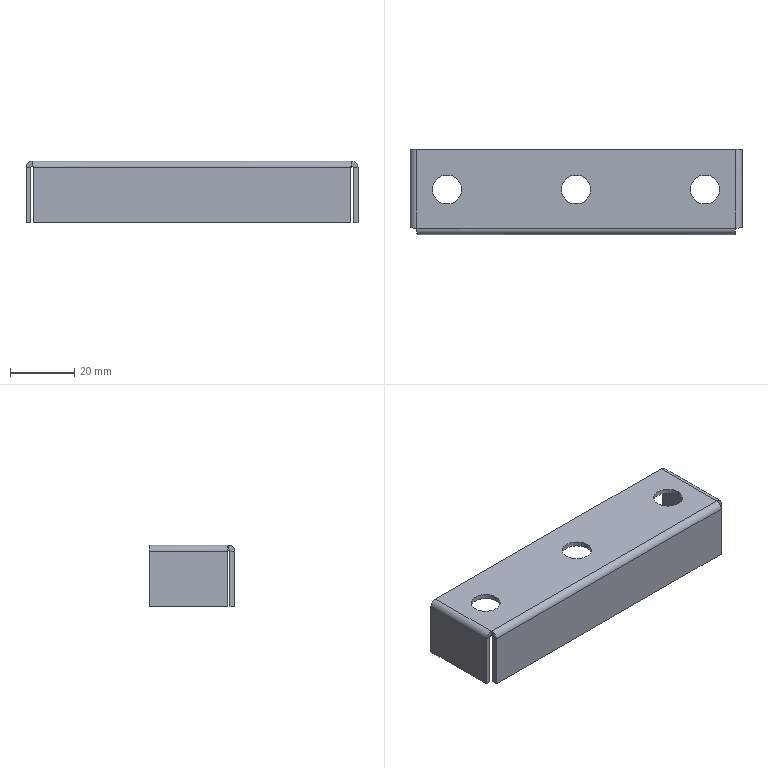Part | SolidWorks | features BaseBody 1 | 1 solid | 36 faces | box 103 x 26.5 x 19.1 mm | volume 7562 mm3 | plane 20 | cylinder 12 | spline 4 | commonest cylinder face diameters 9 x6 1 x3 4 x3
STEP:
#1=CARTESIAN_POINT('',(35.5,0.,-1.5));
#2=VERTEX_POINT('',#1);
#3=CARTESIAN_POINT('',(35.5,0.,0.));
#4=VERTEX_POINT('',#3);
#5=CARTESIAN_POINT('',(35.5,0.,-1.5));
#6=DIRECTION('',(0.,0.,1.));
#7=VECTOR('',#6,1000.);
#8=LINE('',#5,#7);
#9=EDGE_CURVE('',#2,#4,#8,.T.);
#10=ORIENTED_EDGE('',*,*,#9,.F.);
#11=CARTESIAN_POINT('',(44.5,0.,-1.5));
#12=VERTEX_POINT('',#11);
#13=CARTESIAN_POINT('',(40.,0.,-1.5));
#14=DIRECTION('',(0.,0.,1.));
#15=DIRECTION('',(1.,0.,0.));
#16=AXIS2_PLACEMENT_3D('',#13,#14,#15);
#17=CIRCLE('',#16,4.5);
#18=EDGE_CURVE('',#12,#2,#17,.T.);
#19=ORIENTED_EDGE('',*,*,#18,.F.);
#20=CARTESIAN_POINT('',(44.5,0.,0.));
#21=VERTEX_POINT('',#20);
#22=CARTESIAN_POINT('',(44.5,0.,-1.5));
#23=DIRECTION('',(0.,0.,1.));
#24=VECTOR('',#23,1000.);
#25=LINE('',#22,#24);
#26=EDGE_CURVE('',#12,#21,#25,.T.);
#27=ORIENTED_EDGE('',*,*,#26,.T.);
#28=CARTESIAN_POINT('',(40.,0.,0.));
#29=DIRECTION('',(0.,0.,1.));
#30=DIRECTION('',(1.,0.,0.));
#31=AXIS2_PLACEMENT_3D('',#28,#29,#30);
#32=CIRCLE('',#31,4.5);
#33=EDGE_CURVE('',#21,#4,#32,.T.);
#34=ORIENTED_EDGE('',*,*,#33,.T.);
#35=EDGE_LOOP('',(#10,#19,#27,#34));
#36=FACE_OUTER_BOUND('',#35,.T.);
#37=CARTESIAN_POINT('',(40.,0.,-1.5));
#38=DIRECTION('',(0.,0.,1.));
#39=DIRECTION('',(1.,0.,0.));
#40=AXIS2_PLACEMENT_3D('',#37,#38,#39);
#41=CYLINDRICAL_SURFACE('',#40,4.5);
#42=ADVANCED_FACE('',(#36),#41,.F.);
#43=CARTESIAN_POINT('',(-44.5,0.,-1.5));
#44=VERTEX_POINT('',#43);
#45=CARTESIAN_POINT('',(-44.5,0.,0.));
#46=VERTEX_POINT('',#45);
#47=CARTESIAN_POINT('',(-44.5,0.,-1.5));
#48=DIRECTION('',(0.,0.,1.));
#49=VECTOR('',#48,1000.);
#50=LINE('',#47,#49);
#51=EDGE_CURVE('',#44,#46,#50,.T.);
#52=ORIENTED_EDGE('',*,*,#51,.F.);
#53=CARTESIAN_POINT('',(-35.5,0.,-1.5));
#54=VERTEX_POINT('',#53);
#55=CARTESIAN_POINT('',(-40.,0.,-1.5));
#56=DIRECTION('',(0.,0.,1.));
#57=DIRECTION('',(1.,0.,0.));
#58=AXIS2_PLACEMENT_3D('',#55,#56,#57);
#59=CIRCLE('',#58,4.5);
#60=EDGE_CURVE('',#54,#44,#59,.T.);
#61=ORIENTED_EDGE('',*,*,#60,.F.);
#62=CARTESIAN_POINT('',(-35.5,0.,0.));
#63=VERTEX_POINT('',#62);
#64=CARTESIAN_POINT('',(-35.5,0.,-1.5));
#65=DIRECTION('',(0.,0.,1.));
#66=VECTOR('',#65,1000.);
#67=LINE('',#64,#66);
#68=EDGE_CURVE('',#54,#63,#67,.T.);
#69=ORIENTED_EDGE('',*,*,#68,.T.);
#70=CARTESIAN_POINT('',(-40.,0.,0.));
#71=DIRECTION('',(0.,0.,1.));
#72=DIRECTION('',(1.,0.,0.));
#73=AXIS2_PLACEMENT_3D('',#70,#71,#72);
#74=CIRCLE('',#73,4.5);
#75=EDGE_CURVE('',#63,#46,#74,.T.);
#76=ORIENTED_EDGE('',*,*,#75,.T.);
#77=EDGE_LOOP('',(#52,#61,#69,#76));
#78=FACE_OUTER_BOUND('',#77,.T.);
#79=CARTESIAN_POINT('',(-40.,0.,-1.5));
#80=DIRECTION('',(0.,0.,1.));
#81=DIRECTION('',(1.,0.,0.));
#82=AXIS2_PLACEMENT_3D('',#79,#80,#81);
#83=CYLINDRICAL_SURFACE('',#82,4.5);
#84=ADVANCED_FACE('',(#78),#83,.F.);
#85=CARTESIAN_POINT('',(-4.5,0.,-1.5));
#86=VERTEX_POINT('',#85);
#87=CARTESIAN_POINT('',(-4.5,0.,0.));
#88=VERTEX_POINT('',#87);
#89=CARTESIAN_POINT('',(-4.5,0.,-1.5));
#90=DIRECTION('',(0.,0.,1.));
#91=VECTOR('',#90,1000.);
#92=LINE('',#89,#91);
#93=EDGE_CURVE('',#86,#88,#92,.T.);
#94=ORIENTED_EDGE('',*,*,#93,.F.);
#95=CARTESIAN_POINT('',(4.5,0.,-1.5));
#96=VERTEX_POINT('',#95);
#97=CARTESIAN_POINT('',(0.,0.,-1.5));
#98=DIRECTION('',(0.,0.,1.));
#99=DIRECTION('',(1.,0.,0.));
#100=AXIS2_PLACEMENT_3D('',#97,#98,#99);
#101=CIRCLE('',#100,4.5);
#102=EDGE_CURVE('',#96,#86,#101,.T.);
#103=ORIENTED_EDGE('',*,*,#102,.F.);
#104=CARTESIAN_POINT('',(4.5,0.,0.));
#105=VERTEX_POINT('',#104);
#106=CARTESIAN_POINT('',(4.5,0.,-1.5));
#107=DIRECTION('',(0.,0.,1.));
#108=VECTOR('',#107,1000.);
#109=LINE('',#106,#108);
#110=EDGE_CURVE('',#96,#105,#109,.T.);
#111=ORIENTED_EDGE('',*,*,#110,.T.);
#112=CARTESIAN_POINT('',(0.,0.,0.));
#113=DIRECTION('',(0.,0.,1.));
#114=DIRECTION('',(1.,0.,0.));
#115=AXIS2_PLACEMENT_3D('',#112,#113,#114);
#116=CIRCLE('',#115,4.5);
#117=EDGE_CURVE('',#105,#88,#116,.T.);
#118=ORIENTED_EDGE('',*,*,#117,.T.);
#119=EDGE_LOOP('',(#94,#103,#111,#118));
#120=FACE_OUTER_BOUND('',#119,.T.);
#121=CARTESIAN_POINT('',(0.,0.,-1.5));
#122=DIRECTION('',(0.,0.,1.));
#123=DIRECTION('',(1.,0.,0.));
#124=AXIS2_PLACEMENT_3D('',#121,#122,#123);
#125=CYLINDRICAL_SURFACE('',#124,4.5);
#126=ADVANCED_FACE('',(#120),#125,.F.);
#127=CARTESIAN_POINT('',(51.5,-11.793,-19.1));
#128=VERTEX_POINT('',#127);
#129=CARTESIAN_POINT('',(50.,-11.793,-19.1));
#130=VERTEX_POINT('',#129);
#131=CARTESIAN_POINT('',(51.5,-11.793,-19.1));
#132=DIRECTION('',(-1.,0.,0.));
#133=VECTOR('',#132,1000.);
#134=LINE('',#131,#133);
#135=EDGE_CURVE('',#128,#130,#134,.T.);
#136=ORIENTED_EDGE('',*,*,#135,.F.);
#137=CARTESIAN_POINT('',(51.5,-11.793,-2.));
#138=VERTEX_POINT('',#137);
#139=CARTESIAN_POINT('',(51.5,-11.793,0.));
#140=DIRECTION('',(0.,0.,-1.));
#141=VECTOR('',#140,1000.);
#142=LINE('',#139,#141);
#143=EDGE_CURVE('',#138,#128,#142,.T.);
#144=ORIENTED_EDGE('',*,*,#143,.F.);
#145=CARTESIAN_POINT('',(50.,-11.793,-2.));
#146=VERTEX_POINT('',#145);
#147=CARTESIAN_POINT('',(50.,-11.793,-2.));
#148=DIRECTION('',(-1.,0.,0.));
#149=VECTOR('',#148,1000.);
#150=LINE('',#147,#149);
#151=EDGE_CURVE('',#138,#146,#150,.T.);
#152=ORIENTED_EDGE('',*,*,#151,.T.);
#153=CARTESIAN_POINT('',(50.,-11.793,-1.5));
#154=DIRECTION('',(0.,0.,-1.));
#155=VECTOR('',#154,1000.);
#156=LINE('',#153,#155);
#157=EDGE_CURVE('',#146,#130,#156,.T.);
#158=ORIENTED_EDGE('',*,*,#157,.T.);
#159=EDGE_LOOP('',(#136,#144,#152,#158));
#160=FACE_OUTER_BOUND('',#159,.T.);
#161=CARTESIAN_POINT('',(50.,-11.793,-1.5));
#162=DIRECTION('',(0.,1.,0.));
#163=DIRECTION('',(0.,0.,-1.));
#164=AXIS2_PLACEMENT_3D('',#161,#162,#163);
#165=PLANE('',#164);
#166=ADVANCED_FACE('',(#160),#165,.F.);
#167=CARTESIAN_POINT('',(51.5,12.5,-19.1));
#168=VERTEX_POINT('',#167);
#169=CARTESIAN_POINT('',(51.5,12.5,-19.1));
#170=DIRECTION('',(0.,1.,0.));
#171=VECTOR('',#170,1000.);
#172=LINE('',#169,#171);
#173=EDGE_CURVE('',#128,#168,#172,.T.);
#174=ORIENTED_EDGE('',*,*,#173,.F.);
#175=ORIENTED_EDGE('',*,*,#135,.T.);
#176=CARTESIAN_POINT('',(50.,12.5,-19.1));
#177=VERTEX_POINT('',#176);
#178=CARTESIAN_POINT('',(50.,12.5,-19.1));
#179=DIRECTION('',(0.,1.,0.));
#180=VECTOR('',#179,1000.);
#181=LINE('',#178,#180);
#182=EDGE_CURVE('',#130,#177,#181,.T.);
#183=ORIENTED_EDGE('',*,*,#182,.T.);
#184=CARTESIAN_POINT('',(51.5,12.5,-19.1));
#185=DIRECTION('',(-1.,0.,0.));
#186=VECTOR('',#185,1000.);
#187=LINE('',#184,#186);
#188=EDGE_CURVE('',#168,#177,#187,.T.);
#189=ORIENTED_EDGE('',*,*,#188,.F.);
#190=EDGE_LOOP('',(#174,#175,#183,#189));
#191=FACE_OUTER_BOUND('',#190,.T.);
#192=CARTESIAN_POINT('',(51.5,12.5,-19.1));
#193=DIRECTION('',(0.,0.,1.));
#194=DIRECTION('',(1.,0.,0.));
#195=AXIS2_PLACEMENT_3D('',#192,#193,#194);
#196=PLANE('',#195);
#197=ADVANCED_FACE('',(#191),#196,.F.);
#198=ORIENTED_EDGE('',*,*,#157,.F.);
#199=CARTESIAN_POINT('',(50.,12.5,-2.));
#200=VERTEX_POINT('',#199);
#201=CARTESIAN_POINT('',(50.,12.5,-2.));
#202=DIRECTION('',(0.,-1.,0.));
#203=VECTOR('',#202,1000.);
#204=LINE('',#201,#203);
#205=EDGE_CURVE('',#200,#146,#204,.T.);
#206=ORIENTED_EDGE('',*,*,#205,.F.);
#207=CARTESIAN_POINT('',(50.,12.5,-1.5));
#208=DIRECTION('',(0.,0.,1.));
#209=VECTOR('',#208,1000.);
#210=LINE('',#207,#209);
#211=EDGE_CURVE('',#177,#200,#210,.T.);
#212=ORIENTED_EDGE('',*,*,#211,.F.);
#213=ORIENTED_EDGE('',*,*,#182,.F.);
#214=EDGE_LOOP('',(#198,#206,#212,#213));
#215=FACE_OUTER_BOUND('',#214,.T.);
#216=CARTESIAN_POINT('',(50.,0.,0.));
#217=DIRECTION('',(-1.,0.,0.));
#218=DIRECTION('',(0.,0.,1.));
#219=AXIS2_PLACEMENT_3D('',#216,#217,#218);
#220=PLANE('',#219);
#221=ADVANCED_FACE('',(#215),#220,.T.);
#222=CARTESIAN_POINT('',(51.5,12.5,-2.));
#223=VERTEX_POINT('',#222);
#224=CARTESIAN_POINT('',(51.5,0.,-2.));
#225=DIRECTION('',(0.,1.,0.));
#226=VECTOR('',#225,1000.);
#227=LINE('',#224,#226);
#228=EDGE_CURVE('',#138,#223,#227,.T.);
#229=ORIENTED_EDGE('',*,*,#228,.F.);
#230=ORIENTED_EDGE('',*,*,#143,.T.);
#231=ORIENTED_EDGE('',*,*,#173,.T.);
#232=CARTESIAN_POINT('',(51.5,12.5,-1.5));
#233=DIRECTION('',(0.,0.,1.));
#234=VECTOR('',#233,1000.);
#235=LINE('',#232,#234);
#236=EDGE_CURVE('',#168,#223,#235,.T.);
#237=ORIENTED_EDGE('',*,*,#236,.T.);
#238=EDGE_LOOP('',(#229,#230,#231,#237));
#239=FACE_OUTER_BOUND('',#238,.T.);
#240=CARTESIAN_POINT('',(51.5,0.,0.));
#241=DIRECTION('',(-1.,0.,0.));
#242=DIRECTION('',(0.,0.,1.));
#243=AXIS2_PLACEMENT_3D('',#240,#241,#242);
#244=PLANE('',#243);
#245=ADVANCED_FACE('',(#239),#244,.F.);
#246=CARTESIAN_POINT('',(50.,12.5,-2.));
#247=DIRECTION('',(1.,0.,0.));
#248=VECTOR('',#247,1000.);
#249=LINE('',#246,#248);
#250=EDGE_CURVE('',#200,#223,#249,.T.);
#251=ORIENTED_EDGE('',*,*,#250,.T.);
#252=ORIENTED_EDGE('',*,*,#236,.F.);
#253=ORIENTED_EDGE('',*,*,#188,.T.);
#254=ORIENTED_EDGE('',*,*,#211,.T.);
#255=EDGE_LOOP('',(#251,#252,#253,#254));
#256=FACE_OUTER_BOUND('',#255,.T.);
#257=CARTESIAN_POINT('',(51.5,12.5,-1.5));
#258=DIRECTION('',(0.,-1.,0.));
#259=DIRECTION('',(0.,0.,-1.));
#260=AXIS2_PLACEMENT_3D('',#257,#258,#259);
#261=PLANE('',#260);
#262=ADVANCED_FACE('',(#256),#261,.F.);
#263=CARTESIAN_POINT('',(49.5,-12.,-1.5));
#264=VERTEX_POINT('',#263);
#265=CARTESIAN_POINT('',(49.5,12.5,-1.5));
#266=VERTEX_POINT('',#265);
#267=CARTESIAN_POINT('',(49.5,-12.,-1.5));
#268=DIRECTION('',(0.,1.,0.));
#269=VECTOR('',#268,1000.);
#270=LINE('',#267,#269);
#271=EDGE_CURVE('',#264,#266,#270,.T.);
#272=ORIENTED_EDGE('',*,*,#271,.T.);
#273=CARTESIAN_POINT('',(49.5,12.5,-2.));
#274=DIRECTION('',(0.,1.,0.));
#275=DIRECTION('',(0.,0.,-1.));
#276=AXIS2_PLACEMENT_3D('',#273,#274,#275);
#277=CIRCLE('',#276,0.5);
#278=EDGE_CURVE('',#266,#200,#277,.T.);
#279=ORIENTED_EDGE('',*,*,#278,.T.);
#280=ORIENTED_EDGE('',*,*,#205,.T.);
#281=CARTESIAN_POINT('',(50.,-11.793,-2.));
#282=CARTESIAN_POINT('',(50.,-11.827,-1.869));
#283=CARTESIAN_POINT('',(49.946,-11.862,-1.739));
#284=CARTESIAN_POINT('',(49.761,-11.931,-1.554));
#285=CARTESIAN_POINT('',(49.631,-11.965,-1.5));
#286=CARTESIAN_POINT('',(49.5,-12.,-1.5));
#287=B_SPLINE_CURVE_WITH_KNOTS('',3,(#281,#282,#283,#284,#285,#286),.UNSPECIFIED.,.F.,.F.,(4,2,4),(0.,0.5,1.),.UNSPECIFIED.);
#288=EDGE_CURVE('',#146,#264,#287,.T.);
#289=ORIENTED_EDGE('',*,*,#288,.T.);
#290=EDGE_LOOP('',(#272,#279,#280,#289));
#291=FACE_OUTER_BOUND('',#290,.T.);
#292=CARTESIAN_POINT('',(49.5,-12.,-2.));
#293=DIRECTION('',(0.,-1.,0.));
#294=DIRECTION('',(1.,0.,0.));
#295=AXIS2_PLACEMENT_3D('',#292,#293,#294);
#296=CYLINDRICAL_SURFACE('',#295,0.5);
#297=ADVANCED_FACE('',(#291),#296,.F.);
#298=CARTESIAN_POINT('',(49.5,-12.,0.));
#299=VERTEX_POINT('',#298);
#300=CARTESIAN_POINT('',(49.5,12.5,0.));
#301=VERTEX_POINT('',#300);
#302=CARTESIAN_POINT('',(49.5,-12.,0.));
#303=DIRECTION('',(0.,1.,0.));
#304=VECTOR('',#303,1000.);
#305=LINE('',#302,#304);
#306=EDGE_CURVE('',#299,#301,#305,.T.);
#307=ORIENTED_EDGE('',*,*,#306,.F.);
#308=CARTESIAN_POINT('',(51.5,-11.793,-2.));
#309=CARTESIAN_POINT('',(51.5,-11.81,-1.738));
#310=CARTESIAN_POINT('',(51.448,-11.827,-1.477));
#311=CARTESIAN_POINT('',(51.248,-11.862,-0.9928));
#312=CARTESIAN_POINT('',(51.099,-11.879,-0.7709));
#313=CARTESIAN_POINT('',(50.729,-11.914,-0.4007));
#314=CARTESIAN_POINT('',(50.507,-11.931,-0.2524));
#315=CARTESIAN_POINT('',(50.023,-11.965,-0.05205));
#316=CARTESIAN_POINT('',(49.762,-11.983,0.));
#317=CARTESIAN_POINT('',(49.5,-12.,0.));
#318=B_SPLINE_CURVE_WITH_KNOTS('',3,(#308,#309,#310,#311,#312,#313,#314,#315,#316,#317),.UNSPECIFIED.,.F.,.F.,(4,2,2,2,4),(0.,0.25,0.5,0.75,1.),.UNSPECIFIED.);
#319=EDGE_CURVE('',#138,#299,#318,.T.);
#320=ORIENTED_EDGE('',*,*,#319,.F.);
#321=ORIENTED_EDGE('',*,*,#228,.T.);
#322=CARTESIAN_POINT('',(49.5,12.5,-2.));
#323=DIRECTION('',(0.,1.,0.));
#324=DIRECTION('',(0.,0.,-1.));
#325=AXIS2_PLACEMENT_3D('',#322,#323,#324);
#326=CIRCLE('',#325,2.);
#327=EDGE_CURVE('',#301,#223,#326,.T.);
#328=ORIENTED_EDGE('',*,*,#327,.F.);
#329=EDGE_LOOP('',(#307,#320,#321,#328));
#330=FACE_OUTER_BOUND('',#329,.T.);
#331=CARTESIAN_POINT('',(49.5,-12.,-2.));
#332=DIRECTION('',(0.,-1.,0.));
#333=DIRECTION('',(1.,0.,0.));
#334=AXIS2_PLACEMENT_3D('',#331,#332,#333);
#335=CYLINDRICAL_SURFACE('',#334,2.);
#336=ADVANCED_FACE('',(#330),#335,.T.);
#337=ORIENTED_EDGE('',*,*,#288,.F.);
#338=ORIENTED_EDGE('',*,*,#151,.F.);
#339=ORIENTED_EDGE('',*,*,#319,.T.);
#340=CARTESIAN_POINT('',(49.5,-12.,-1.5));
#341=DIRECTION('',(0.,0.,1.));
#342=VECTOR('',#341,1000.);
#343=LINE('',#340,#342);
#344=EDGE_CURVE('',#264,#299,#343,.T.);
#345=ORIENTED_EDGE('',*,*,#344,.F.);
#346=EDGE_LOOP('',(#337,#338,#339,#345));
#347=FACE_OUTER_BOUND('',#346,.T.);
#348=CARTESIAN_POINT('',(51.515,-11.793,-2.));
#349=CARTESIAN_POINT('',(51.515,-11.81,-1.736));
#350=CARTESIAN_POINT('',(51.463,-11.827,-1.473));
#351=CARTESIAN_POINT('',(51.261,-11.862,-0.9852));
#352=CARTESIAN_POINT('',(51.111,-11.879,-0.7617));
#353=CARTESIAN_POINT('',(50.738,-11.914,-0.3887));
#354=CARTESIAN_POINT('',(50.515,-11.931,-0.2393));
#355=CARTESIAN_POINT('',(50.027,-11.965,-0.03745));
#356=CARTESIAN_POINT('',(49.764,-11.983,0.015));
#357=CARTESIAN_POINT('',(49.5,-12.,0.015));
#358=CARTESIAN_POINT('',(51.5,-11.793,-2.));
#359=CARTESIAN_POINT('',(51.5,-11.81,-1.738));
#360=CARTESIAN_POINT('',(51.448,-11.827,-1.477));
#361=CARTESIAN_POINT('',(51.248,-11.862,-0.9928));
#362=CARTESIAN_POINT('',(51.099,-11.879,-0.7709));
#363=CARTESIAN_POINT('',(50.729,-11.914,-0.4007));
#364=CARTESIAN_POINT('',(50.507,-11.931,-0.2524));
#365=CARTESIAN_POINT('',(50.023,-11.965,-0.05205));
#366=CARTESIAN_POINT('',(49.762,-11.983,0.));
#367=CARTESIAN_POINT('',(49.5,-12.,0.));
#368=CARTESIAN_POINT('',(50.,-11.793,-2.));
#369=CARTESIAN_POINT('',(50.,-11.81,-1.935));
#370=CARTESIAN_POINT('',(49.987,-11.827,-1.869));
#371=CARTESIAN_POINT('',(49.937,-11.862,-1.748));
#372=CARTESIAN_POINT('',(49.9,-11.879,-1.693));
#373=CARTESIAN_POINT('',(49.807,-11.914,-1.6));
#374=CARTESIAN_POINT('',(49.752,-11.931,-1.563));
#375=CARTESIAN_POINT('',(49.631,-11.965,-1.513));
#376=CARTESIAN_POINT('',(49.565,-11.983,-1.5));
#377=CARTESIAN_POINT('',(49.5,-12.,-1.5));
#378=CARTESIAN_POINT('',(49.985,-11.793,-2.));
#379=CARTESIAN_POINT('',(49.985,-11.81,-1.937));
#380=CARTESIAN_POINT('',(49.972,-11.827,-1.873));
#381=CARTESIAN_POINT('',(49.924,-11.862,-1.756));
#382=CARTESIAN_POINT('',(49.888,-11.879,-1.702));
#383=CARTESIAN_POINT('',(49.798,-11.914,-1.612));
#384=CARTESIAN_POINT('',(49.744,-11.931,-1.576));
#385=CARTESIAN_POINT('',(49.627,-11.965,-1.528));
#386=CARTESIAN_POINT('',(49.563,-11.983,-1.515));
#387=CARTESIAN_POINT('',(49.5,-12.,-1.515));
#388=B_SPLINE_SURFACE_WITH_KNOTS('',1,3,((#348,#349,#350,#351,#352,#353,#354,#355,#356,#357),(#358,#359,#360,#361,#362,#363,#364,#365,#366,#367),(#368,#369,#370,#371,#372,#373,#374,#375,#376,#377),(#378,#379,#380,#381,#382,#383,#384,#385,#386,#387)),.UNSPECIFIED.,.F.,.F.,.F.,(2,1,1,2),(4,2,2,2,4),(-0.01,0.,1.,1.01),(0.,0.25,0.5,0.75,1.),.UNSPECIFIED.);
#389=ADVANCED_FACE('',(#347),#388,.F.);
#390=ORIENTED_EDGE('',*,*,#250,.F.);
#391=ORIENTED_EDGE('',*,*,#278,.F.);
#392=CARTESIAN_POINT('',(49.5,12.5,-1.5));
#393=DIRECTION('',(0.,0.,1.));
#394=VECTOR('',#393,1000.);
#395=LINE('',#392,#394);
#396=EDGE_CURVE('',#266,#301,#395,.T.);
#397=ORIENTED_EDGE('',*,*,#396,.T.);
#398=ORIENTED_EDGE('',*,*,#327,.T.);
#399=EDGE_LOOP('',(#390,#391,#397,#398));
#400=FACE_OUTER_BOUND('',#399,.T.);
#401=CARTESIAN_POINT('',(49.5,12.5,-2.));
#402=DIRECTION('',(0.,1.,0.));
#403=DIRECTION('',(1.,0.,0.));
#404=AXIS2_PLACEMENT_3D('',#401,#402,#403);
#405=PLANE('',#404);
#406=ADVANCED_FACE('',(#400),#405,.T.);
#407=CARTESIAN_POINT('',(-49.293,-14.,-19.1));
#408=VERTEX_POINT('',#407);
#409=CARTESIAN_POINT('',(-49.293,-12.5,-19.1));
#410=VERTEX_POINT('',#409);
#411=CARTESIAN_POINT('',(-49.293,-14.,-19.1));
#412=DIRECTION('',(0.,1.,0.));
#413=VECTOR('',#412,1000.);
#414=LINE('',#411,#413);
#415=EDGE_CURVE('',#408,#410,#414,.T.);
#416=ORIENTED_EDGE('',*,*,#415,.F.);
#417=CARTESIAN_POINT('',(-49.293,-14.,-2.));
#418=VERTEX_POINT('',#417);
#419=CARTESIAN_POINT('',(-49.293,-14.,0.));
#420=DIRECTION('',(0.,0.,-1.));
#421=VECTOR('',#420,1000.);
#422=LINE('',#419,#421);
#423=EDGE_CURVE('',#418,#408,#422,.T.);
#424=ORIENTED_EDGE('',*,*,#423,.F.);
#425=CARTESIAN_POINT('',(-49.293,-12.5,-2.));
#426=VERTEX_POINT('',#425);
#427=CARTESIAN_POINT('',(-49.293,-12.5,-2.));
#428=DIRECTION('',(0.,1.,0.));
#429=VECTOR('',#428,1000.);
#430=LINE('',#427,#429);
#431=EDGE_CURVE('',#418,#426,#430,.T.);
#432=ORIENTED_EDGE('',*,*,#431,.T.);
#433=CARTESIAN_POINT('',(-49.293,-12.5,-1.5));
#434=DIRECTION('',(0.,0.,-1.));
#435=VECTOR('',#434,1000.);
#436=LINE('',#433,#435);
#437=EDGE_CURVE('',#426,#410,#436,.T.);
#438=ORIENTED_EDGE('',*,*,#437,.T.);
#439=EDGE_LOOP('',(#416,#424,#432,#438));
#440=FACE_OUTER_BOUND('',#439,.T.);
#441=CARTESIAN_POINT('',(-49.293,-12.5,-1.5));
#442=DIRECTION('',(1.,0.,0.));
#443=DIRECTION('',(0.,1.,0.));
#444=AXIS2_PLACEMENT_3D('',#441,#442,#443);
#445=PLANE('',#444);
#446=ADVANCED_FACE('',(#440),#445,.F.);
#447=CARTESIAN_POINT('',(49.293,-14.,-19.1));
#448=VERTEX_POINT('',#447);
#449=CARTESIAN_POINT('',(49.293,-12.5,-19.1));
#450=VERTEX_POINT('',#449);
#451=CARTESIAN_POINT('',(49.293,-14.,-19.1));
#452=DIRECTION('',(0.,1.,0.));
#453=VECTOR('',#452,1000.);
#454=LINE('',#451,#453);
#455=EDGE_CURVE('',#448,#450,#454,.T.);
#456=ORIENTED_EDGE('',*,*,#455,.F.);
#457=CARTESIAN_POINT('',(50.,-14.,-19.1));
#458=DIRECTION('',(1.,0.,0.));
#459=VECTOR('',#458,1000.);
#460=LINE('',#457,#459);
#461=EDGE_CURVE('',#408,#448,#460,.T.);
#462=ORIENTED_EDGE('',*,*,#461,.F.);
#463=ORIENTED_EDGE('',*,*,#415,.T.);
#464=CARTESIAN_POINT('',(50.,-12.5,-19.1));
#465=DIRECTION('',(1.,0.,0.));
#466=VECTOR('',#465,1000.);
#467=LINE('',#464,#466);
#468=EDGE_CURVE('',#410,#450,#467,.T.);
#469=ORIENTED_EDGE('',*,*,#468,.T.);
#470=EDGE_LOOP('',(#456,#462,#463,#469));
#471=FACE_OUTER_BOUND('',#470,.T.);
#472=CARTESIAN_POINT('',(50.,-14.,-19.1));
#473=DIRECTION('',(0.,0.,1.));
#474=DIRECTION('',(0.,-1.,0.));
#475=AXIS2_PLACEMENT_3D('',#472,#473,#474);
#476=PLANE('',#475);
#477=ADVANCED_FACE('',(#471),#476,.F.);
#478=CARTESIAN_POINT('',(49.293,-12.5,-2.));
#479=VERTEX_POINT('',#478);
#480=CARTESIAN_POINT('',(50.,-12.5,-2.));
#481=DIRECTION('',(-1.,0.,0.));
#482=VECTOR('',#481,1000.);
#483=LINE('',#480,#482);
#484=EDGE_CURVE('',#479,#426,#483,.T.);
#485=ORIENTED_EDGE('',*,*,#484,.F.);
#486=CARTESIAN_POINT('',(49.293,-12.5,-1.5));
#487=DIRECTION('',(0.,0.,-1.));
#488=VECTOR('',#487,1000.);
#489=LINE('',#486,#488);
#490=EDGE_CURVE('',#479,#450,#489,.T.);
#491=ORIENTED_EDGE('',*,*,#490,.T.);
#492=ORIENTED_EDGE('',*,*,#468,.F.);
#493=ORIENTED_EDGE('',*,*,#437,.F.);
#494=EDGE_LOOP('',(#485,#491,#492,#493));
#495=FACE_OUTER_BOUND('',#494,.T.);
#496=CARTESIAN_POINT('',(0.,-12.5,0.));
#497=DIRECTION('',(0.,1.,0.));
#498=DIRECTION('',(0.,0.,-1.));
#499=AXIS2_PLACEMENT_3D('',#496,#497,#498);
#500=PLANE('',#499);
#501=ADVANCED_FACE('',(#495),#500,.T.);
#502=CARTESIAN_POINT('',(49.293,-14.,-2.));
#503=VERTEX_POINT('',#502);
#504=CARTESIAN_POINT('',(49.293,-14.,0.));
#505=DIRECTION('',(0.,0.,-1.));
#506=VECTOR('',#505,1000.);
#507=LINE('',#504,#506);
#508=EDGE_CURVE('',#503,#448,#507,.T.);
#509=ORIENTED_EDGE('',*,*,#508,.F.);
#510=CARTESIAN_POINT('',(0.,-14.,-2.));
#511=DIRECTION('',(1.,0.,0.));
#512=VECTOR('',#511,1000.);
#513=LINE('',#510,#512);
#514=EDGE_CURVE('',#418,#503,#513,.T.);
#515=ORIENTED_EDGE('',*,*,#514,.F.);
#516=ORIENTED_EDGE('',*,*,#423,.T.);
#517=ORIENTED_EDGE('',*,*,#461,.T.);
#518=EDGE_LOOP('',(#509,#515,#516,#517));
#519=FACE_OUTER_BOUND('',#518,.T.);
#520=CARTESIAN_POINT('',(0.,-14.,0.));
#521=DIRECTION('',(0.,1.,0.));
#522=DIRECTION('',(0.,0.,-1.));
#523=AXIS2_PLACEMENT_3D('',#520,#521,#522);
#524=PLANE('',#523);
#525=ADVANCED_FACE('',(#519),#524,.F.);
#526=ORIENTED_EDGE('',*,*,#508,.T.);
#527=ORIENTED_EDGE('',*,*,#455,.T.);
#528=ORIENTED_EDGE('',*,*,#490,.F.);
#529=CARTESIAN_POINT('',(49.293,-12.5,-2.));
#530=DIRECTION('',(0.,1.,0.));
#531=VECTOR('',#530,1000.);
#532=LINE('',#529,#531);
#533=EDGE_CURVE('',#503,#479,#532,.T.);
#534=ORIENTED_EDGE('',*,*,#533,.F.);
#535=EDGE_LOOP('',(#526,#527,#528,#534));
#536=FACE_OUTER_BOUND('',#535,.T.);
#537=CARTESIAN_POINT('',(49.293,-12.5,-1.5));
#538=DIRECTION('',(1.,0.,0.));
#539=DIRECTION('',(0.,1.,0.));
#540=AXIS2_PLACEMENT_3D('',#537,#538,#539);
#541=PLANE('',#540);
#542=ADVANCED_FACE('',(#536),#541,.T.);
#543=CARTESIAN_POINT('',(-49.5,-12.,-1.5));
#544=VERTEX_POINT('',#543);
#545=CARTESIAN_POINT('',(-49.5,-12.,-1.5));
#546=DIRECTION('',(1.,0.,0.));
#547=VECTOR('',#546,1000.);
#548=LINE('',#545,#547);
#549=EDGE_CURVE('',#544,#264,#548,.T.);
#550=ORIENTED_EDGE('',*,*,#549,.T.);
#551=CARTESIAN_POINT('',(49.5,-12.,-1.5));
#552=CARTESIAN_POINT('',(49.465,-12.131,-1.5));
#553=CARTESIAN_POINT('',(49.431,-12.261,-1.554));
#554=CARTESIAN_POINT('',(49.362,-12.446,-1.739));
#555=CARTESIAN_POINT('',(49.327,-12.5,-1.869));
#556=CARTESIAN_POINT('',(49.293,-12.5,-2.));
#557=B_SPLINE_CURVE_WITH_KNOTS('',3,(#551,#552,#553,#554,#555,#556),.UNSPECIFIED.,.F.,.F.,(4,2,4),(0.,0.5,1.),.UNSPECIFIED.);
#558=EDGE_CURVE('',#264,#479,#557,.T.);
#559=ORIENTED_EDGE('',*,*,#558,.T.);
#560=ORIENTED_EDGE('',*,*,#484,.T.);
#561=CARTESIAN_POINT('',(-49.293,-12.5,-2.));
#562=CARTESIAN_POINT('',(-49.327,-12.5,-1.869));
#563=CARTESIAN_POINT('',(-49.362,-12.446,-1.739));
#564=CARTESIAN_POINT('',(-49.431,-12.261,-1.554));
#565=CARTESIAN_POINT('',(-49.465,-12.131,-1.5));
#566=CARTESIAN_POINT('',(-49.5,-12.,-1.5));
#567=B_SPLINE_CURVE_WITH_KNOTS('',3,(#561,#562,#563,#564,#565,#566),.UNSPECIFIED.,.F.,.F.,(4,2,4),(0.,0.5,1.),.UNSPECIFIED.);
#568=EDGE_CURVE('',#426,#544,#567,.T.);
#569=ORIENTED_EDGE('',*,*,#568,.T.);
#570=EDGE_LOOP('',(#550,#559,#560,#569));
#571=FACE_OUTER_BOUND('',#570,.T.);
#572=CARTESIAN_POINT('',(-49.5,-12.,-2.));
#573=DIRECTION('',(-1.,0.,0.));
#574=DIRECTION('',(0.,-1.,0.));
#575=AXIS2_PLACEMENT_3D('',#572,#573,#574);
#576=CYLINDRICAL_SURFACE('',#575,0.5);
#577=ADVANCED_FACE('',(#571),#576,.F.);
#578=CARTESIAN_POINT('',(-49.5,-12.,0.));
#579=VERTEX_POINT('',#578);
#580=CARTESIAN_POINT('',(-49.5,-12.,0.));
#581=DIRECTION('',(1.,0.,0.));
#582=VECTOR('',#581,1000.);
#583=LINE('',#580,#582);
#584=EDGE_CURVE('',#579,#299,#583,.T.);
#585=ORIENTED_EDGE('',*,*,#584,.F.);
#586=CARTESIAN_POINT('',(-49.293,-14.,-2.));
#587=CARTESIAN_POINT('',(-49.31,-14.,-1.738));
#588=CARTESIAN_POINT('',(-49.327,-13.948,-1.477));
#589=CARTESIAN_POINT('',(-49.362,-13.748,-0.9928));
#590=CARTESIAN_POINT('',(-49.379,-13.599,-0.7709));
#591=CARTESIAN_POINT('',(-49.414,-13.229,-0.4007));
#592=CARTESIAN_POINT('',(-49.431,-13.007,-0.2524));
#593=CARTESIAN_POINT('',(-49.465,-12.523,-0.05205));
#594=CARTESIAN_POINT('',(-49.483,-12.262,0.));
#595=CARTESIAN_POINT('',(-49.5,-12.,0.));
#596=B_SPLINE_CURVE_WITH_KNOTS('',3,(#586,#587,#588,#589,#590,#591,#592,#593,#594,#595),.UNSPECIFIED.,.F.,.F.,(4,2,2,2,4),(0.,0.25,0.5,0.75,1.),.UNSPECIFIED.);
#597=EDGE_CURVE('',#418,#579,#596,.T.);
#598=ORIENTED_EDGE('',*,*,#597,.F.);
#599=ORIENTED_EDGE('',*,*,#514,.T.);
#600=CARTESIAN_POINT('',(49.5,-12.,0.));
#601=CARTESIAN_POINT('',(49.483,-12.262,0.));
#602=CARTESIAN_POINT('',(49.465,-12.523,-0.05205));
#603=CARTESIAN_POINT('',(49.431,-13.007,-0.2524));
#604=CARTESIAN_POINT('',(49.414,-13.229,-0.4007));
#605=CARTESIAN_POINT('',(49.379,-13.599,-0.7709));
#606=CARTESIAN_POINT('',(49.362,-13.748,-0.9928));
#607=CARTESIAN_POINT('',(49.327,-13.948,-1.477));
#608=CARTESIAN_POINT('',(49.31,-14.,-1.738));
#609=CARTESIAN_POINT('',(49.293,-14.,-2.));
#610=B_SPLINE_CURVE_WITH_KNOTS('',3,(#600,#601,#602,#603,#604,#605,#606,#607,#608,#609),.UNSPECIFIED.,.F.,.F.,(4,2,2,2,4),(0.,0.25,0.5,0.75,1.),.UNSPECIFIED.);
#611=EDGE_CURVE('',#299,#503,#610,.T.);
#612=ORIENTED_EDGE('',*,*,#611,.F.);
#613=EDGE_LOOP('',(#585,#598,#599,#612));
#614=FACE_OUTER_BOUND('',#613,.T.);
#615=CARTESIAN_POINT('',(-49.5,-12.,-2.));
#616=DIRECTION('',(-1.,0.,0.));
#617=DIRECTION('',(0.,-1.,0.));
#618=AXIS2_PLACEMENT_3D('',#615,#616,#617);
#619=CYLINDRICAL_SURFACE('',#618,2.);
#620=ADVANCED_FACE('',(#614),#619,.T.);
#621=ORIENTED_EDGE('',*,*,#568,.F.);
#622=ORIENTED_EDGE('',*,*,#431,.F.);
#623=ORIENTED_EDGE('',*,*,#597,.T.);
#624=CARTESIAN_POINT('',(-49.5,-12.,-1.5));
#625=DIRECTION('',(0.,0.,1.));
#626=VECTOR('',#625,1000.);
#627=LINE('',#624,#626);
#628=EDGE_CURVE('',#544,#579,#627,.T.);
#629=ORIENTED_EDGE('',*,*,#628,.F.);
#630=EDGE_LOOP('',(#621,#622,#623,#629));
#631=FACE_OUTER_BOUND('',#630,.T.);
#632=CARTESIAN_POINT('',(-49.293,-14.015,-2.));
#633=CARTESIAN_POINT('',(-49.31,-14.015,-1.736));
#634=CARTESIAN_POINT('',(-49.327,-13.963,-1.473));
#635=CARTESIAN_POINT('',(-49.362,-13.761,-0.9852));
#636=CARTESIAN_POINT('',(-49.379,-13.611,-0.7617));
#637=CARTESIAN_POINT('',(-49.414,-13.238,-0.3887));
#638=CARTESIAN_POINT('',(-49.431,-13.015,-0.2393));
#639=CARTESIAN_POINT('',(-49.465,-12.527,-0.03745));
#640=CARTESIAN_POINT('',(-49.483,-12.264,0.015));
#641=CARTESIAN_POINT('',(-49.5,-12.,0.015));
#642=CARTESIAN_POINT('',(-49.293,-14.,-2.));
#643=CARTESIAN_POINT('',(-49.31,-14.,-1.738));
#644=CARTESIAN_POINT('',(-49.327,-13.948,-1.477));
#645=CARTESIAN_POINT('',(-49.362,-13.748,-0.9928));
#646=CARTESIAN_POINT('',(-49.379,-13.599,-0.7709));
#647=CARTESIAN_POINT('',(-49.414,-13.229,-0.4007));
#648=CARTESIAN_POINT('',(-49.431,-13.007,-0.2524));
#649=CARTESIAN_POINT('',(-49.465,-12.523,-0.05205));
#650=CARTESIAN_POINT('',(-49.483,-12.262,0.));
#651=CARTESIAN_POINT('',(-49.5,-12.,0.));
#652=CARTESIAN_POINT('',(-49.293,-12.5,-2.));
#653=CARTESIAN_POINT('',(-49.31,-12.5,-1.935));
#654=CARTESIAN_POINT('',(-49.327,-12.487,-1.869));
#655=CARTESIAN_POINT('',(-49.362,-12.437,-1.748));
#656=CARTESIAN_POINT('',(-49.379,-12.4,-1.693));
#657=CARTESIAN_POINT('',(-49.414,-12.307,-1.6));
#658=CARTESIAN_POINT('',(-49.431,-12.252,-1.563));
#659=CARTESIAN_POINT('',(-49.465,-12.131,-1.513));
#660=CARTESIAN_POINT('',(-49.483,-12.065,-1.5));
#661=CARTESIAN_POINT('',(-49.5,-12.,-1.5));
#662=CARTESIAN_POINT('',(-49.293,-12.485,-2.));
#663=CARTESIAN_POINT('',(-49.31,-12.485,-1.937));
#664=CARTESIAN_POINT('',(-49.327,-12.472,-1.873));
#665=CARTESIAN_POINT('',(-49.362,-12.424,-1.756));
#666=CARTESIAN_POINT('',(-49.379,-12.388,-1.702));
#667=CARTESIAN_POINT('',(-49.414,-12.298,-1.612));
#668=CARTESIAN_POINT('',(-49.431,-12.244,-1.576));
#669=CARTESIAN_POINT('',(-49.465,-12.127,-1.528));
#670=CARTESIAN_POINT('',(-49.483,-12.063,-1.515));
#671=CARTESIAN_POINT('',(-49.5,-12.,-1.515));
#672=B_SPLINE_SURFACE_WITH_KNOTS('',1,3,((#632,#633,#634,#635,#636,#637,#638,#639,#640,#641),(#642,#643,#644,#645,#646,#647,#648,#649,#650,#651),(#652,#653,#654,#655,#656,#657,#658,#659,#660,#661),(#662,#663,#664,#665,#666,#667,#668,#669,#670,#671)),.UNSPECIFIED.,.F.,.F.,.F.,(2,1,1,2),(4,2,2,2,4),(-0.01,0.,1.,1.01),(0.,0.25,0.5,0.75,1.),.UNSPECIFIED.);
#673=ADVANCED_FACE('',(#631),#672,.F.);
#674=ORIENTED_EDGE('',*,*,#533,.T.);
#675=ORIENTED_EDGE('',*,*,#558,.F.);
#676=ORIENTED_EDGE('',*,*,#344,.T.);
#677=ORIENTED_EDGE('',*,*,#611,.T.);
#678=EDGE_LOOP('',(#674,#675,#676,#677));
#679=FACE_OUTER_BOUND('',#678,.T.);
#680=CARTESIAN_POINT('',(49.5,-12.,0.015));
#681=CARTESIAN_POINT('',(49.483,-12.264,0.015));
#682=CARTESIAN_POINT('',(49.465,-12.527,-0.03745));
#683=CARTESIAN_POINT('',(49.431,-13.015,-0.2393));
#684=CARTESIAN_POINT('',(49.414,-13.238,-0.3887));
#685=CARTESIAN_POINT('',(49.379,-13.611,-0.7617));
#686=CARTESIAN_POINT('',(49.362,-13.761,-0.9852));
#687=CARTESIAN_POINT('',(49.327,-13.963,-1.473));
#688=CARTESIAN_POINT('',(49.31,-14.015,-1.736));
#689=CARTESIAN_POINT('',(49.293,-14.015,-2.));
#690=CARTESIAN_POINT('',(49.5,-12.,0.));
#691=CARTESIAN_POINT('',(49.483,-12.262,0.));
#692=CARTESIAN_POINT('',(49.465,-12.523,-0.05205));
#693=CARTESIAN_POINT('',(49.431,-13.007,-0.2524));
#694=CARTESIAN_POINT('',(49.414,-13.229,-0.4007));
#695=CARTESIAN_POINT('',(49.379,-13.599,-0.7709));
#696=CARTESIAN_POINT('',(49.362,-13.748,-0.9928));
#697=CARTESIAN_POINT('',(49.327,-13.948,-1.477));
#698=CARTESIAN_POINT('',(49.31,-14.,-1.738));
#699=CARTESIAN_POINT('',(49.293,-14.,-2.));
#700=CARTESIAN_POINT('',(49.5,-12.,-1.5));
#701=CARTESIAN_POINT('',(49.483,-12.065,-1.5));
#702=CARTESIAN_POINT('',(49.465,-12.131,-1.513));
#703=CARTESIAN_POINT('',(49.431,-12.252,-1.563));
#704=CARTESIAN_POINT('',(49.414,-12.307,-1.6));
#705=CARTESIAN_POINT('',(49.379,-12.4,-1.693));
#706=CARTESIAN_POINT('',(49.362,-12.437,-1.748));
#707=CARTESIAN_POINT('',(49.327,-12.487,-1.869));
#708=CARTESIAN_POINT('',(49.31,-12.5,-1.935));
#709=CARTESIAN_POINT('',(49.293,-12.5,-2.));
#710=CARTESIAN_POINT('',(49.5,-12.,-1.515));
#711=CARTESIAN_POINT('',(49.483,-12.063,-1.515));
#712=CARTESIAN_POINT('',(49.465,-12.127,-1.528));
#713=CARTESIAN_POINT('',(49.431,-12.244,-1.576));
#714=CARTESIAN_POINT('',(49.414,-12.298,-1.612));
#715=CARTESIAN_POINT('',(49.379,-12.388,-1.702));
#716=CARTESIAN_POINT('',(49.362,-12.424,-1.756));
#717=CARTESIAN_POINT('',(49.327,-12.472,-1.873));
#718=CARTESIAN_POINT('',(49.31,-12.485,-1.937));
#719=CARTESIAN_POINT('',(49.293,-12.485,-2.));
#720=B_SPLINE_SURFACE_WITH_KNOTS('',1,3,((#680,#681,#682,#683,#684,#685,#686,#687,#688,#689),(#690,#691,#692,#693,#694,#695,#696,#697,#698,#699),(#700,#701,#702,#703,#704,#705,#706,#707,#708,#709),(#710,#711,#712,#713,#714,#715,#716,#717,#718,#719)),.UNSPECIFIED.,.F.,.F.,.F.,(2,1,1,2),(4,2,2,2,4),(-0.01,0.,1.,1.01),(0.,0.25,0.5,0.75,1.),.UNSPECIFIED.);
#721=ADVANCED_FACE('',(#679),#720,.F.);
#722=CARTESIAN_POINT('',(-50.,12.5,-2.));
#723=VERTEX_POINT('',#722);
#724=CARTESIAN_POINT('',(-51.5,12.5,-2.));
#725=VERTEX_POINT('',#724);
#726=CARTESIAN_POINT('',(-50.,12.5,-2.));
#727=DIRECTION('',(-1.,0.,0.));
#728=VECTOR('',#727,1000.);
#729=LINE('',#726,#728);
#730=EDGE_CURVE('',#723,#725,#729,.T.);
#731=ORIENTED_EDGE('',*,*,#730,.F.);
#732=CARTESIAN_POINT('',(-50.,12.5,-19.1));
#733=VERTEX_POINT('',#732);
#734=CARTESIAN_POINT('',(-50.,12.5,-19.1));
#735=DIRECTION('',(0.,0.,-1.));
#736=VECTOR('',#735,1000.);
#737=LINE('',#734,#736);
#738=EDGE_CURVE('',#723,#733,#737,.T.);
#739=ORIENTED_EDGE('',*,*,#738,.T.);
#740=CARTESIAN_POINT('',(-51.5,12.5,-19.1));
#741=VERTEX_POINT('',#740);
#742=CARTESIAN_POINT('',(-51.5,12.5,-19.1));
#743=DIRECTION('',(1.,0.,0.));
#744=VECTOR('',#743,1000.);
#745=LINE('',#742,#744);
#746=EDGE_CURVE('',#741,#733,#745,.T.);
#747=ORIENTED_EDGE('',*,*,#746,.F.);
#748=CARTESIAN_POINT('',(-51.5,12.5,-19.1));
#749=DIRECTION('',(0.,0.,-1.));
#750=VECTOR('',#749,1000.);
#751=LINE('',#748,#750);
#752=EDGE_CURVE('',#725,#741,#751,.T.);
#753=ORIENTED_EDGE('',*,*,#752,.F.);
#754=EDGE_LOOP('',(#731,#739,#747,#753));
#755=FACE_OUTER_BOUND('',#754,.T.);
#756=CARTESIAN_POINT('',(-51.5,12.5,-19.1));
#757=DIRECTION('',(0.,-1.,0.));
#758=DIRECTION('',(-1.,0.,0.));
#759=AXIS2_PLACEMENT_3D('',#756,#757,#758);
#760=PLANE('',#759);
#761=ADVANCED_FACE('',(#755),#760,.F.);
#762=CARTESIAN_POINT('',(-51.5,-11.793,-19.1));
#763=VERTEX_POINT('',#762);
#764=CARTESIAN_POINT('',(-50.,-11.793,-19.1));
#765=VERTEX_POINT('',#764);
#766=CARTESIAN_POINT('',(-51.5,-11.793,-19.1));
#767=DIRECTION('',(1.,0.,0.));
#768=VECTOR('',#767,1000.);
#769=LINE('',#766,#768);
#770=EDGE_CURVE('',#763,#765,#769,.T.);
#771=ORIENTED_EDGE('',*,*,#770,.F.);
#772=CARTESIAN_POINT('',(-51.5,-12.5,-19.1));
#773=DIRECTION('',(0.,-1.,0.));
#774=VECTOR('',#773,1000.);
#775=LINE('',#772,#774);
#776=EDGE_CURVE('',#741,#763,#775,.T.);
#777=ORIENTED_EDGE('',*,*,#776,.F.);
#778=ORIENTED_EDGE('',*,*,#746,.T.);
#779=CARTESIAN_POINT('',(-50.,-12.5,-19.1));
#780=DIRECTION('',(0.,-1.,0.));
#781=VECTOR('',#780,1000.);
#782=LINE('',#779,#781);
#783=EDGE_CURVE('',#733,#765,#782,.T.);
#784=ORIENTED_EDGE('',*,*,#783,.T.);
#785=EDGE_LOOP('',(#771,#777,#778,#784));
#786=FACE_OUTER_BOUND('',#785,.T.);
#787=CARTESIAN_POINT('',(-51.5,-12.5,-19.1));
#788=DIRECTION('',(0.,0.,1.));
#789=DIRECTION('',(1.,0.,0.));
#790=AXIS2_PLACEMENT_3D('',#787,#788,#789);
#791=PLANE('',#790);
#792=ADVANCED_FACE('',(#786),#791,.F.);
#793=CARTESIAN_POINT('',(-50.,-11.793,-2.));
#794=VERTEX_POINT('',#793);
#795=CARTESIAN_POINT('',(-50.,-12.5,-2.));
#796=DIRECTION('',(0.,1.,0.));
#797=VECTOR('',#796,1000.);
#798=LINE('',#795,#797);
#799=EDGE_CURVE('',#794,#723,#798,.T.);
#800=ORIENTED_EDGE('',*,*,#799,.F.);
#801=CARTESIAN_POINT('',(-50.,-11.793,-1.5));
#802=DIRECTION('',(0.,0.,-1.));
#803=VECTOR('',#802,1000.);
#804=LINE('',#801,#803);
#805=EDGE_CURVE('',#794,#765,#804,.T.);
#806=ORIENTED_EDGE('',*,*,#805,.T.);
#807=ORIENTED_EDGE('',*,*,#783,.F.);
#808=ORIENTED_EDGE('',*,*,#738,.F.);
#809=EDGE_LOOP('',(#800,#806,#807,#808));
#810=FACE_OUTER_BOUND('',#809,.T.);
#811=CARTESIAN_POINT('',(-50.,0.,0.));
#812=DIRECTION('',(1.,0.,0.));
#813=DIRECTION('',(0.,0.,-1.));
#814=AXIS2_PLACEMENT_3D('',#811,#812,#813);
#815=PLANE('',#814);
#816=ADVANCED_FACE('',(#810),#815,.T.);
#817=CARTESIAN_POINT('',(-51.5,-11.793,-2.));
#818=VERTEX_POINT('',#817);
#819=CARTESIAN_POINT('',(-51.5,-11.793,0.));
#820=DIRECTION('',(0.,0.,-1.));
#821=VECTOR('',#820,1000.);
#822=LINE('',#819,#821);
#823=EDGE_CURVE('',#818,#763,#822,.T.);
#824=ORIENTED_EDGE('',*,*,#823,.F.);
#825=CARTESIAN_POINT('',(-51.5,0.,-2.));
#826=DIRECTION('',(0.,-1.,0.));
#827=VECTOR('',#826,1000.);
#828=LINE('',#825,#827);
#829=EDGE_CURVE('',#725,#818,#828,.T.);
#830=ORIENTED_EDGE('',*,*,#829,.F.);
#831=ORIENTED_EDGE('',*,*,#752,.T.);
#832=ORIENTED_EDGE('',*,*,#776,.T.);
#833=EDGE_LOOP('',(#824,#830,#831,#832));
#834=FACE_OUTER_BOUND('',#833,.T.);
#835=CARTESIAN_POINT('',(-51.5,0.,0.));
#836=DIRECTION('',(1.,0.,0.));
#837=DIRECTION('',(0.,0.,-1.));
#838=AXIS2_PLACEMENT_3D('',#835,#836,#837);
#839=PLANE('',#838);
#840=ADVANCED_FACE('',(#834),#839,.F.);
#841=ORIENTED_EDGE('',*,*,#823,.T.);
#842=ORIENTED_EDGE('',*,*,#770,.T.);
#843=ORIENTED_EDGE('',*,*,#805,.F.);
#844=CARTESIAN_POINT('',(-50.,-11.793,-2.));
#845=DIRECTION('',(1.,0.,0.));
#846=VECTOR('',#845,1000.);
#847=LINE('',#844,#846);
#848=EDGE_CURVE('',#818,#794,#847,.T.);
#849=ORIENTED_EDGE('',*,*,#848,.F.);
#850=EDGE_LOOP('',(#841,#842,#843,#849));
#851=FACE_OUTER_BOUND('',#850,.T.);
#852=CARTESIAN_POINT('',(-50.,-11.793,-1.5));
#853=DIRECTION('',(0.,-1.,0.));
#854=DIRECTION('',(0.,0.,-1.));
#855=AXIS2_PLACEMENT_3D('',#852,#853,#854);
#856=PLANE('',#855);
#857=ADVANCED_FACE('',(#851),#856,.T.);
#858=CARTESIAN_POINT('',(-49.5,12.5,-1.5));
#859=VERTEX_POINT('',#858);
#860=CARTESIAN_POINT('',(-49.5,12.5,-1.5));
#861=DIRECTION('',(0.,-1.,0.));
#862=VECTOR('',#861,1000.);
#863=LINE('',#860,#862);
#864=EDGE_CURVE('',#859,#544,#863,.T.);
#865=ORIENTED_EDGE('',*,*,#864,.T.);
#866=CARTESIAN_POINT('',(-49.5,-12.,-1.5));
#867=CARTESIAN_POINT('',(-49.631,-11.965,-1.5));
#868=CARTESIAN_POINT('',(-49.761,-11.931,-1.554));
#869=CARTESIAN_POINT('',(-49.946,-11.862,-1.739));
#870=CARTESIAN_POINT('',(-50.,-11.827,-1.869));
#871=CARTESIAN_POINT('',(-50.,-11.793,-2.));
#872=B_SPLINE_CURVE_WITH_KNOTS('',3,(#866,#867,#868,#869,#870,#871),.UNSPECIFIED.,.F.,.F.,(4,2,4),(0.,0.5,1.),.UNSPECIFIED.);
#873=EDGE_CURVE('',#544,#794,#872,.T.);
#874=ORIENTED_EDGE('',*,*,#873,.T.);
#875=ORIENTED_EDGE('',*,*,#799,.T.);
#876=CARTESIAN_POINT('',(-49.5,12.5,-2.));
#877=DIRECTION('',(0.,1.,0.));
#878=DIRECTION('',(0.,0.,1.));
#879=AXIS2_PLACEMENT_3D('',#876,#877,#878);
#880=CIRCLE('',#879,0.5);
#881=EDGE_CURVE('',#723,#859,#880,.T.);
#882=ORIENTED_EDGE('',*,*,#881,.T.);
#883=EDGE_LOOP('',(#865,#874,#875,#882));
#884=FACE_OUTER_BOUND('',#883,.T.);
#885=CARTESIAN_POINT('',(-49.5,12.5,-2.));
#886=DIRECTION('',(0.,1.,0.));
#887=DIRECTION('',(-1.,0.,0.));
#888=AXIS2_PLACEMENT_3D('',#885,#886,#887);
#889=CYLINDRICAL_SURFACE('',#888,0.5);
#890=ADVANCED_FACE('',(#884),#889,.F.);
#891=CARTESIAN_POINT('',(-49.5,12.5,0.));
#892=VERTEX_POINT('',#891);
#893=CARTESIAN_POINT('',(-49.5,12.5,0.));
#894=DIRECTION('',(0.,-1.,0.));
#895=VECTOR('',#894,1000.);
#896=LINE('',#893,#895);
#897=EDGE_CURVE('',#892,#579,#896,.T.);
#898=ORIENTED_EDGE('',*,*,#897,.F.);
#899=CARTESIAN_POINT('',(-49.5,12.5,-2.));
#900=DIRECTION('',(0.,1.,0.));
#901=DIRECTION('',(0.,0.,1.));
#902=AXIS2_PLACEMENT_3D('',#899,#900,#901);
#903=CIRCLE('',#902,2.);
#904=EDGE_CURVE('',#725,#892,#903,.T.);
#905=ORIENTED_EDGE('',*,*,#904,.F.);
#906=ORIENTED_EDGE('',*,*,#829,.T.);
#907=CARTESIAN_POINT('',(-49.5,-12.,0.));
#908=CARTESIAN_POINT('',(-49.762,-11.983,0.));
#909=CARTESIAN_POINT('',(-50.023,-11.965,-0.05205));
#910=CARTESIAN_POINT('',(-50.507,-11.931,-0.2524));
#911=CARTESIAN_POINT('',(-50.729,-11.914,-0.4007));
#912=CARTESIAN_POINT('',(-51.099,-11.879,-0.7709));
#913=CARTESIAN_POINT('',(-51.248,-11.862,-0.9928));
#914=CARTESIAN_POINT('',(-51.448,-11.827,-1.477));
#915=CARTESIAN_POINT('',(-51.5,-11.81,-1.738));
#916=CARTESIAN_POINT('',(-51.5,-11.793,-2.));
#917=B_SPLINE_CURVE_WITH_KNOTS('',3,(#907,#908,#909,#910,#911,#912,#913,#914,#915,#916),.UNSPECIFIED.,.F.,.F.,(4,2,2,2,4),(0.,0.25,0.5,0.75,1.),.UNSPECIFIED.);
#918=EDGE_CURVE('',#579,#818,#917,.T.);
#919=ORIENTED_EDGE('',*,*,#918,.F.);
#920=EDGE_LOOP('',(#898,#905,#906,#919));
#921=FACE_OUTER_BOUND('',#920,.T.);
#922=CARTESIAN_POINT('',(-49.5,12.5,-2.));
#923=DIRECTION('',(0.,1.,0.));
#924=DIRECTION('',(-1.,0.,0.));
#925=AXIS2_PLACEMENT_3D('',#922,#923,#924);
#926=CYLINDRICAL_SURFACE('',#925,2.);
#927=ADVANCED_FACE('',(#921),#926,.T.);
#928=ORIENTED_EDGE('',*,*,#881,.F.);
#929=ORIENTED_EDGE('',*,*,#730,.T.);
#930=ORIENTED_EDGE('',*,*,#904,.T.);
#931=CARTESIAN_POINT('',(-49.5,12.5,-1.5));
#932=DIRECTION('',(0.,0.,1.));
#933=VECTOR('',#932,1000.);
#934=LINE('',#931,#933);
#935=EDGE_CURVE('',#859,#892,#934,.T.);
#936=ORIENTED_EDGE('',*,*,#935,.F.);
#937=EDGE_LOOP('',(#928,#929,#930,#936));
#938=FACE_OUTER_BOUND('',#937,.T.);
#939=CARTESIAN_POINT('',(-49.5,12.5,-2.));
#940=DIRECTION('',(0.,-1.,0.));
#941=DIRECTION('',(0.,0.,-1.));
#942=AXIS2_PLACEMENT_3D('',#939,#940,#941);
#943=PLANE('',#942);
#944=ADVANCED_FACE('',(#938),#943,.F.);
#945=ORIENTED_EDGE('',*,*,#848,.T.);
#946=ORIENTED_EDGE('',*,*,#873,.F.);
#947=ORIENTED_EDGE('',*,*,#628,.T.);
#948=ORIENTED_EDGE('',*,*,#918,.T.);
#949=EDGE_LOOP('',(#945,#946,#947,#948));
#950=FACE_OUTER_BOUND('',#949,.T.);
#951=CARTESIAN_POINT('',(-49.5,-12.,0.015));
#952=CARTESIAN_POINT('',(-49.764,-11.983,0.015));
#953=CARTESIAN_POINT('',(-50.027,-11.965,-0.03745));
#954=CARTESIAN_POINT('',(-50.515,-11.931,-0.2393));
#955=CARTESIAN_POINT('',(-50.738,-11.914,-0.3887));
#956=CARTESIAN_POINT('',(-51.111,-11.879,-0.7617));
#957=CARTESIAN_POINT('',(-51.261,-11.862,-0.9852));
#958=CARTESIAN_POINT('',(-51.463,-11.827,-1.473));
#959=CARTESIAN_POINT('',(-51.515,-11.81,-1.736));
#960=CARTESIAN_POINT('',(-51.515,-11.793,-2.));
#961=CARTESIAN_POINT('',(-49.5,-12.,0.));
#962=CARTESIAN_POINT('',(-49.762,-11.983,0.));
#963=CARTESIAN_POINT('',(-50.023,-11.965,-0.05205));
#964=CARTESIAN_POINT('',(-50.507,-11.931,-0.2524));
#965=CARTESIAN_POINT('',(-50.729,-11.914,-0.4007));
#966=CARTESIAN_POINT('',(-51.099,-11.879,-0.7709));
#967=CARTESIAN_POINT('',(-51.248,-11.862,-0.9928));
#968=CARTESIAN_POINT('',(-51.448,-11.827,-1.477));
#969=CARTESIAN_POINT('',(-51.5,-11.81,-1.738));
#970=CARTESIAN_POINT('',(-51.5,-11.793,-2.));
#971=CARTESIAN_POINT('',(-49.5,-12.,-1.5));
#972=CARTESIAN_POINT('',(-49.565,-11.983,-1.5));
#973=CARTESIAN_POINT('',(-49.631,-11.965,-1.513));
#974=CARTESIAN_POINT('',(-49.752,-11.931,-1.563));
#975=CARTESIAN_POINT('',(-49.807,-11.914,-1.6));
#976=CARTESIAN_POINT('',(-49.9,-11.879,-1.693));
#977=CARTESIAN_POINT('',(-49.937,-11.862,-1.748));
#978=CARTESIAN_POINT('',(-49.987,-11.827,-1.869));
#979=CARTESIAN_POINT('',(-50.,-11.81,-1.935));
#980=CARTESIAN_POINT('',(-50.,-11.793,-2.));
#981=CARTESIAN_POINT('',(-49.5,-12.,-1.515));
#982=CARTESIAN_POINT('',(-49.563,-11.983,-1.515));
#983=CARTESIAN_POINT('',(-49.627,-11.965,-1.528));
#984=CARTESIAN_POINT('',(-49.744,-11.931,-1.576));
#985=CARTESIAN_POINT('',(-49.798,-11.914,-1.612));
#986=CARTESIAN_POINT('',(-49.888,-11.879,-1.702));
#987=CARTESIAN_POINT('',(-49.924,-11.862,-1.756));
#988=CARTESIAN_POINT('',(-49.972,-11.827,-1.873));
#989=CARTESIAN_POINT('',(-49.985,-11.81,-1.937));
#990=CARTESIAN_POINT('',(-49.985,-11.793,-2.));
#991=B_SPLINE_SURFACE_WITH_KNOTS('',1,3,((#951,#952,#953,#954,#955,#956,#957,#958,#959,#960),(#961,#962,#963,#964,#965,#966,#967,#968,#969,#970),(#971,#972,#973,#974,#975,#976,#977,#978,#979,#980),(#981,#982,#983,#984,#985,#986,#987,#988,#989,#990)),.UNSPECIFIED.,.F.,.F.,.F.,(2,1,1,2),(4,2,2,2,4),(-0.01,0.,1.,1.01),(0.,0.25,0.5,0.75,1.),.UNSPECIFIED.);
#992=ADVANCED_FACE('',(#950),#991,.F.);
#993=ORIENTED_EDGE('',*,*,#396,.F.);
#994=CARTESIAN_POINT('',(50.,12.5,-1.5));
#995=DIRECTION('',(-1.,0.,0.));
#996=VECTOR('',#995,1000.);
#997=LINE('',#994,#996);
#998=EDGE_CURVE('',#266,#859,#997,.T.);
#999=ORIENTED_EDGE('',*,*,#998,.T.);
#1000=ORIENTED_EDGE('',*,*,#935,.T.);
#1001=CARTESIAN_POINT('',(50.,12.5,0.));
#1002=DIRECTION('',(-1.,0.,0.));
#1003=VECTOR('',#1002,1000.);
#1004=LINE('',#1001,#1003);
#1005=EDGE_CURVE('',#301,#892,#1004,.T.);
#1006=ORIENTED_EDGE('',*,*,#1005,.F.);
#1007=EDGE_LOOP('',(#993,#999,#1000,#1006));
#1008=FACE_OUTER_BOUND('',#1007,.T.);
#1009=CARTESIAN_POINT('',(50.,12.5,-1.5));
#1010=DIRECTION('',(0.,1.,0.));
#1011=DIRECTION('',(1.,0.,0.));
#1012=AXIS2_PLACEMENT_3D('',#1009,#1010,#1011);
#1013=PLANE('',#1012);
#1014=ADVANCED_FACE('',(#1008),#1013,.T.);
#1015=ORIENTED_EDGE('',*,*,#117,.F.);
#1016=CARTESIAN_POINT('',(0.,0.,0.));
#1017=DIRECTION('',(0.,0.,1.));
#1018=DIRECTION('',(1.,0.,0.));
#1019=AXIS2_PLACEMENT_3D('',#1016,#1017,#1018);
#1020=CIRCLE('',#1019,4.5);
#1021=EDGE_CURVE('',#88,#105,#1020,.T.);
#1022=ORIENTED_EDGE('',*,*,#1021,.F.);
#1023=EDGE_LOOP('',(#1015,#1022));
#1024=FACE_BOUND('',#1023,.T.);
#1025=ORIENTED_EDGE('',*,*,#75,.F.);
#1026=CARTESIAN_POINT('',(-40.,0.,0.));
#1027=DIRECTION('',(0.,0.,1.));
#1028=DIRECTION('',(1.,0.,0.));
#1029=AXIS2_PLACEMENT_3D('',#1026,#1027,#1028);
#1030=CIRCLE('',#1029,4.5);
#1031=EDGE_CURVE('',#46,#63,#1030,.T.);
#1032=ORIENTED_EDGE('',*,*,#1031,.F.);
#1033=EDGE_LOOP('',(#1025,#1032));
#1034=FACE_BOUND('',#1033,.T.);
#1035=ORIENTED_EDGE('',*,*,#33,.F.);
#1036=CARTESIAN_POINT('',(40.,0.,0.));
#1037=DIRECTION('',(0.,0.,1.));
#1038=DIRECTION('',(1.,0.,0.));
#1039=AXIS2_PLACEMENT_3D('',#1036,#1037,#1038);
#1040=CIRCLE('',#1039,4.5);
#1041=EDGE_CURVE('',#4,#21,#1040,.T.);
#1042=ORIENTED_EDGE('',*,*,#1041,.F.);
#1043=EDGE_LOOP('',(#1035,#1042));
#1044=FACE_BOUND('',#1043,.T.);
#1045=ORIENTED_EDGE('',*,*,#306,.T.);
#1046=ORIENTED_EDGE('',*,*,#1005,.T.);
#1047=ORIENTED_EDGE('',*,*,#897,.T.);
#1048=ORIENTED_EDGE('',*,*,#584,.T.);
#1049=EDGE_LOOP('',(#1045,#1046,#1047,#1048));
#1050=FACE_OUTER_BOUND('',#1049,.T.);
#1051=CARTESIAN_POINT('',(0.,0.,0.));
#1052=DIRECTION('',(0.,0.,-1.));
#1053=DIRECTION('',(0.,-1.,0.));
#1054=AXIS2_PLACEMENT_3D('',#1051,#1052,#1053);
#1055=PLANE('',#1054);
#1056=ADVANCED_FACE('',(#1024,#1034,#1044,#1050),#1055,.F.);
#1057=ORIENTED_EDGE('',*,*,#102,.T.);
#1058=CARTESIAN_POINT('',(0.,0.,-1.5));
#1059=DIRECTION('',(0.,0.,1.));
#1060=DIRECTION('',(1.,0.,0.));
#1061=AXIS2_PLACEMENT_3D('',#1058,#1059,#1060);
#1062=CIRCLE('',#1061,4.5);
#1063=EDGE_CURVE('',#86,#96,#1062,.T.);
#1064=ORIENTED_EDGE('',*,*,#1063,.T.);
#1065=EDGE_LOOP('',(#1057,#1064));
#1066=FACE_BOUND('',#1065,.T.);
#1067=ORIENTED_EDGE('',*,*,#60,.T.);
#1068=CARTESIAN_POINT('',(-40.,0.,-1.5));
#1069=DIRECTION('',(0.,0.,1.));
#1070=DIRECTION('',(1.,0.,0.));
#1071=AXIS2_PLACEMENT_3D('',#1068,#1069,#1070);
#1072=CIRCLE('',#1071,4.5);
#1073=EDGE_CURVE('',#44,#54,#1072,.T.);
#1074=ORIENTED_EDGE('',*,*,#1073,.T.);
#1075=EDGE_LOOP('',(#1067,#1074));
#1076=FACE_BOUND('',#1075,.T.);
#1077=ORIENTED_EDGE('',*,*,#18,.T.);
#1078=CARTESIAN_POINT('',(40.,0.,-1.5));
#1079=DIRECTION('',(0.,0.,1.));
#1080=DIRECTION('',(1.,0.,0.));
#1081=AXIS2_PLACEMENT_3D('',#1078,#1079,#1080);
#1082=CIRCLE('',#1081,4.5);
#1083=EDGE_CURVE('',#2,#12,#1082,.T.);
#1084=ORIENTED_EDGE('',*,*,#1083,.T.);
#1085=EDGE_LOOP('',(#1077,#1084));
#1086=FACE_BOUND('',#1085,.T.);
#1087=ORIENTED_EDGE('',*,*,#998,.F.);
#1088=ORIENTED_EDGE('',*,*,#271,.F.);
#1089=ORIENTED_EDGE('',*,*,#549,.F.);
#1090=ORIENTED_EDGE('',*,*,#864,.F.);
#1091=EDGE_LOOP('',(#1087,#1088,#1089,#1090));
#1092=FACE_OUTER_BOUND('',#1091,.T.);
#1093=CARTESIAN_POINT('',(0.,0.,-1.5));
#1094=DIRECTION('',(0.,0.,-1.));
#1095=DIRECTION('',(0.,-1.,0.));
#1096=AXIS2_PLACEMENT_3D('',#1093,#1094,#1095);
#1097=PLANE('',#1096);
#1098=ADVANCED_FACE('',(#1066,#1076,#1086,#1092),#1097,.T.);
#1099=ORIENTED_EDGE('',*,*,#1063,.F.);
#1100=ORIENTED_EDGE('',*,*,#93,.T.);
#1101=ORIENTED_EDGE('',*,*,#1021,.T.);
#1102=ORIENTED_EDGE('',*,*,#110,.F.);
#1103=EDGE_LOOP('',(#1099,#1100,#1101,#1102));
#1104=FACE_OUTER_BOUND('',#1103,.T.);
#1105=CARTESIAN_POINT('',(0.,0.,-1.5));
#1106=DIRECTION('',(0.,0.,1.));
#1107=DIRECTION('',(1.,0.,0.));
#1108=AXIS2_PLACEMENT_3D('',#1105,#1106,#1107);
#1109=CYLINDRICAL_SURFACE('',#1108,4.5);
#1110=ADVANCED_FACE('',(#1104),#1109,.F.);
#1111=ORIENTED_EDGE('',*,*,#1073,.F.);
#1112=ORIENTED_EDGE('',*,*,#51,.T.);
#1113=ORIENTED_EDGE('',*,*,#1031,.T.);
#1114=ORIENTED_EDGE('',*,*,#68,.F.);
#1115=EDGE_LOOP('',(#1111,#1112,#1113,#1114));
#1116=FACE_OUTER_BOUND('',#1115,.T.);
#1117=CARTESIAN_POINT('',(-40.,0.,-1.5));
#1118=DIRECTION('',(0.,0.,1.));
#1119=DIRECTION('',(1.,0.,0.));
#1120=AXIS2_PLACEMENT_3D('',#1117,#1118,#1119);
#1121=CYLINDRICAL_SURFACE('',#1120,4.5);
#1122=ADVANCED_FACE('',(#1116),#1121,.F.);
#1123=ORIENTED_EDGE('',*,*,#1083,.F.);
#1124=ORIENTED_EDGE('',*,*,#9,.T.);
#1125=ORIENTED_EDGE('',*,*,#1041,.T.);
#1126=ORIENTED_EDGE('',*,*,#26,.F.);
#1127=EDGE_LOOP('',(#1123,#1124,#1125,#1126));
#1128=FACE_OUTER_BOUND('',#1127,.T.);
#1129=CARTESIAN_POINT('',(40.,0.,-1.5));
#1130=DIRECTION('',(0.,0.,1.));
#1131=DIRECTION('',(1.,0.,0.));
#1132=AXIS2_PLACEMENT_3D('',#1129,#1130,#1131);
#1133=CYLINDRICAL_SURFACE('',#1132,4.5);
#1134=ADVANCED_FACE('',(#1128),#1133,.F.);
#1135=CLOSED_SHELL('',(#42,#84,#126,#166,#197,#221,#245,#262,#297,#336,#389,#406,#446,#477,#501,#525,#542,#577,#620,#673,#721,#761,#792,#816,#840,#857,#890,#927,#944,#992,#1014,#1056,#1098,#1110,#1122,#1134));
#1136=MANIFOLD_SOLID_BREP('',#1135);
#1137=CARTESIAN_POINT('',(0.,0.,0.));
#1138=DIRECTION('',(0.,0.,1.));
#1139=DIRECTION('',(1.,0.,0.));
#1140=AXIS2_PLACEMENT_3D('',#1137,#1138,#1139);
#1141=(LENGTH_UNIT()NAMED_UNIT(*)SI_UNIT(.MILLI.,.METRE.));
#1142=UNCERTAINTY_MEASURE_WITH_UNIT(LENGTH_MEASURE(0.00001),#1141,'','');
#1143=(NAMED_UNIT(*)PLANE_ANGLE_UNIT()SI_UNIT($,.RADIAN.));
#1144=(NAMED_UNIT(*)SI_UNIT($,.STERADIAN.)SOLID_ANGLE_UNIT());
#1145=(GEOMETRIC_REPRESENTATION_CONTEXT(3)GLOBAL_UNCERTAINTY_ASSIGNED_CONTEXT((#1142))GLOBAL_UNIT_ASSIGNED_CONTEXT((#1141,#1143,#1144))REPRESENTATION_CONTEXT('',''));
#1146=ADVANCED_BREP_SHAPE_REPRESENTATION('',(#1136,#1140),#1145);